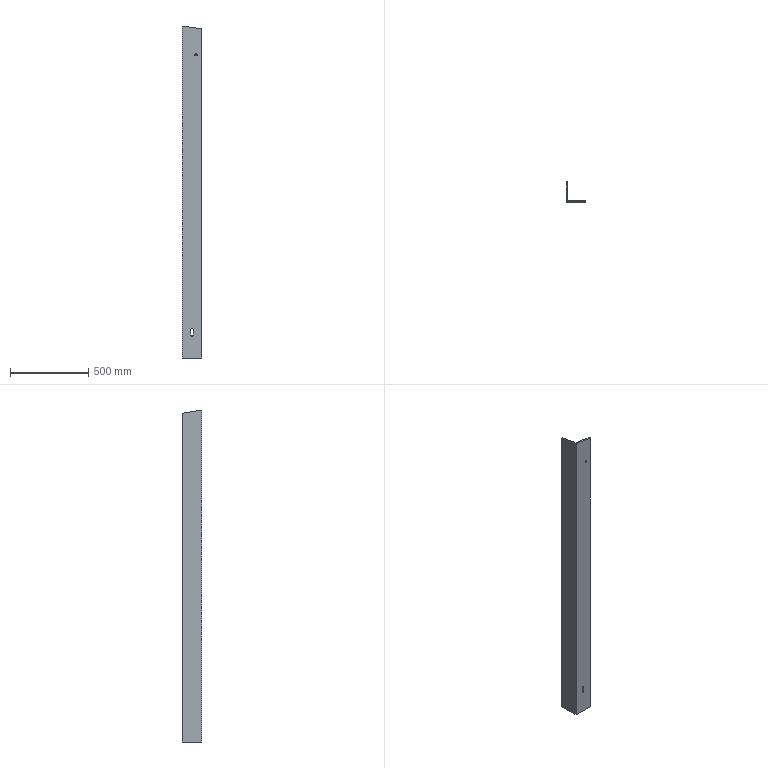Part | SolidWorks | features ICE 2, Extrusion 1 | 1 solid | 15 faces | box 127 x 127 x 2128 mm | volume 4129005 mm3 | plane 11 | cylinder 4 | commonest cylinder face diameters 14.287 x4
STEP:
#1=CARTESIAN_POINT('',(96.044,0.,879.284));
#2=VERTEX_POINT('',#1);
#3=CARTESIAN_POINT('',(81.756,0.,879.284));
#4=VERTEX_POINT('',#3);
#5=CARTESIAN_POINT('',(88.9,0.,879.284));
#6=DIRECTION('',(0.,1.,0.));
#7=DIRECTION('',(0.,0.,1.));
#8=AXIS2_PLACEMENT_3D('',#5,#6,#7);
#9=CIRCLE('',#8,7.144);
#10=EDGE_CURVE('',#2,#4,#9,.T.);
#11=ORIENTED_EDGE('',*,*,#10,.F.);
#12=CARTESIAN_POINT('',(96.044,7.937,879.284));
#13=VERTEX_POINT('',#12);
#14=CARTESIAN_POINT('',(96.044,-242.062,879.284));
#15=DIRECTION('',(0.,1.,0.));
#16=VECTOR('',#15,1000.);
#17=LINE('',#14,#16);
#18=EDGE_CURVE('',#2,#13,#17,.T.);
#19=ORIENTED_EDGE('',*,*,#18,.T.);
#20=CARTESIAN_POINT('',(81.756,7.937,879.284));
#21=VERTEX_POINT('',#20);
#22=CARTESIAN_POINT('',(88.9,7.937,879.284));
#23=DIRECTION('',(0.,-1.,0.));
#24=DIRECTION('',(1.,0.,0.));
#25=AXIS2_PLACEMENT_3D('',#22,#23,#24);
#26=CIRCLE('',#25,7.144);
#27=EDGE_CURVE('',#21,#13,#26,.T.);
#28=ORIENTED_EDGE('',*,*,#27,.F.);
#29=CARTESIAN_POINT('',(81.756,-242.062,879.284));
#30=DIRECTION('',(0.,1.,0.));
#31=VECTOR('',#30,1000.);
#32=LINE('',#29,#31);
#33=EDGE_CURVE('',#4,#21,#32,.T.);
#34=ORIENTED_EDGE('',*,*,#33,.F.);
#35=EDGE_LOOP('',(#11,#19,#28,#34));
#36=FACE_OUTER_BOUND('',#35,.T.);
#37=CARTESIAN_POINT('',(88.9,-242.062,879.284));
#38=DIRECTION('',(0.,1.,0.));
#39=DIRECTION('',(-1.,0.,0.));
#40=AXIS2_PLACEMENT_3D('',#37,#38,#39);
#41=CYLINDRICAL_SURFACE('',#40,7.144);
#42=ADVANCED_FACE('',(#36),#41,.F.);
#43=CARTESIAN_POINT('',(0.,127.,1042.677));
#44=VERTEX_POINT('',#43);
#45=CARTESIAN_POINT('',(0.,127.,-1063.815));
#46=VERTEX_POINT('',#45);
#47=CARTESIAN_POINT('',(0.,127.,1063.815));
#48=DIRECTION('',(0.,0.,-1.));
#49=VECTOR('',#48,1000.);
#50=LINE('',#47,#49);
#51=EDGE_CURVE('',#44,#46,#50,.T.);
#52=ORIENTED_EDGE('',*,*,#51,.F.);
#53=CARTESIAN_POINT('',(7.938,127.,1042.677));
#54=VERTEX_POINT('',#53);
#55=CARTESIAN_POINT('',(150.,127.,1042.677));
#56=DIRECTION('',(-1.,0.,0.));
#57=VECTOR('',#56,1000.);
#58=LINE('',#55,#57);
#59=EDGE_CURVE('',#54,#44,#58,.T.);
#60=ORIENTED_EDGE('',*,*,#59,.F.);
#61=CARTESIAN_POINT('',(7.938,127.,-1063.815));
#62=VERTEX_POINT('',#61);
#63=CARTESIAN_POINT('',(7.938,127.,1063.815));
#64=DIRECTION('',(0.,0.,-1.));
#65=VECTOR('',#64,1000.);
#66=LINE('',#63,#65);
#67=EDGE_CURVE('',#54,#62,#66,.T.);
#68=ORIENTED_EDGE('',*,*,#67,.T.);
#69=CARTESIAN_POINT('',(7.938,127.,-1063.815));
#70=DIRECTION('',(-1.,0.,0.));
#71=VECTOR('',#70,1000.);
#72=LINE('',#69,#71);
#73=EDGE_CURVE('',#62,#46,#72,.T.);
#74=ORIENTED_EDGE('',*,*,#73,.T.);
#75=EDGE_LOOP('',(#52,#60,#68,#74));
#76=FACE_OUTER_BOUND('',#75,.T.);
#77=CARTESIAN_POINT('',(7.938,127.,1063.815));
#78=DIRECTION('',(0.,-1.,0.));
#79=DIRECTION('',(0.,0.,-1.));
#80=AXIS2_PLACEMENT_3D('',#77,#78,#79);
#81=PLANE('',#80);
#82=ADVANCED_FACE('',(#76),#81,.F.);
#83=CARTESIAN_POINT('',(0.,0.,1063.815));
#84=VERTEX_POINT('',#83);
#85=CARTESIAN_POINT('',(0.,0.,-1063.815));
#86=VERTEX_POINT('',#85);
#87=CARTESIAN_POINT('',(0.,0.,1063.815));
#88=DIRECTION('',(0.,0.,-1.));
#89=VECTOR('',#88,1000.);
#90=LINE('',#87,#89);
#91=EDGE_CURVE('',#84,#86,#90,.T.);
#92=ORIENTED_EDGE('',*,*,#91,.F.);
#93=CARTESIAN_POINT('',(0.,0.,1063.815));
#94=DIRECTION('',(0.,-0.9864,0.1642));
#95=VECTOR('',#94,1000.);
#96=LINE('',#93,#95);
#97=EDGE_CURVE('',#44,#84,#96,.T.);
#98=ORIENTED_EDGE('',*,*,#97,.F.);
#99=ORIENTED_EDGE('',*,*,#51,.T.);
#100=CARTESIAN_POINT('',(0.,127.,-1063.815));
#101=DIRECTION('',(0.,-1.,0.));
#102=VECTOR('',#101,1000.);
#103=LINE('',#100,#102);
#104=EDGE_CURVE('',#46,#86,#103,.T.);
#105=ORIENTED_EDGE('',*,*,#104,.T.);
#106=EDGE_LOOP('',(#92,#98,#99,#105));
#107=FACE_OUTER_BOUND('',#106,.T.);
#108=CARTESIAN_POINT('',(0.,127.,1063.815));
#109=DIRECTION('',(1.,0.,0.));
#110=DIRECTION('',(0.,0.,-1.));
#111=AXIS2_PLACEMENT_3D('',#108,#109,#110);
#112=PLANE('',#111);
#113=ADVANCED_FACE('',(#107),#112,.F.);
#114=CARTESIAN_POINT('',(88.9,0.,879.284));
#115=DIRECTION('',(0.,1.,0.));
#116=DIRECTION('',(0.,0.,1.));
#117=AXIS2_PLACEMENT_3D('',#114,#115,#116);
#118=CIRCLE('',#117,7.144);
#119=EDGE_CURVE('',#4,#2,#118,.T.);
#120=ORIENTED_EDGE('',*,*,#119,.T.);
#121=ORIENTED_EDGE('',*,*,#10,.T.);
#122=EDGE_LOOP('',(#120,#121));
#123=FACE_BOUND('',#122,.T.);
#124=CARTESIAN_POINT('',(70.644,0.,-880.459));
#125=VERTEX_POINT('',#124);
#126=CARTESIAN_POINT('',(70.644,0.,-916.972));
#127=VERTEX_POINT('',#126);
#128=CARTESIAN_POINT('',(70.644,0.,1063.815));
#129=DIRECTION('',(0.,0.,-1.));
#130=VECTOR('',#129,1000.);
#131=LINE('',#128,#130);
#132=EDGE_CURVE('',#125,#127,#131,.T.);
#133=ORIENTED_EDGE('',*,*,#132,.T.);
#134=CARTESIAN_POINT('',(56.356,0.,-916.972));
#135=VERTEX_POINT('',#134);
#136=CARTESIAN_POINT('',(63.5,0.,-916.972));
#137=DIRECTION('',(0.,1.,0.));
#138=DIRECTION('',(0.,0.,1.));
#139=AXIS2_PLACEMENT_3D('',#136,#137,#138);
#140=CIRCLE('',#139,7.144);
#141=EDGE_CURVE('',#127,#135,#140,.T.);
#142=ORIENTED_EDGE('',*,*,#141,.T.);
#143=CARTESIAN_POINT('',(56.356,0.,-880.459));
#144=VERTEX_POINT('',#143);
#145=CARTESIAN_POINT('',(56.356,0.,1063.815));
#146=DIRECTION('',(0.,0.,1.));
#147=VECTOR('',#146,1000.);
#148=LINE('',#145,#147);
#149=EDGE_CURVE('',#135,#144,#148,.T.);
#150=ORIENTED_EDGE('',*,*,#149,.T.);
#151=CARTESIAN_POINT('',(63.5,0.,-880.459));
#152=DIRECTION('',(0.,1.,0.));
#153=DIRECTION('',(0.,0.,1.));
#154=AXIS2_PLACEMENT_3D('',#151,#152,#153);
#155=CIRCLE('',#154,7.144);
#156=EDGE_CURVE('',#144,#125,#155,.T.);
#157=ORIENTED_EDGE('',*,*,#156,.T.);
#158=EDGE_LOOP('',(#133,#142,#150,#157));
#159=FACE_BOUND('',#158,.T.);
#160=CARTESIAN_POINT('',(127.,0.,1045.56));
#161=VERTEX_POINT('',#160);
#162=CARTESIAN_POINT('',(127.,0.,-1063.815));
#163=VERTEX_POINT('',#162);
#164=CARTESIAN_POINT('',(127.,0.,1063.815));
#165=DIRECTION('',(0.,0.,-1.));
#166=VECTOR('',#165,1000.);
#167=LINE('',#164,#166);
#168=EDGE_CURVE('',#161,#163,#167,.T.);
#169=ORIENTED_EDGE('',*,*,#168,.F.);
#170=CARTESIAN_POINT('',(0.,0.,1063.815));
#171=DIRECTION('',(-0.9898,0.,0.1423));
#172=VECTOR('',#171,1000.);
#173=LINE('',#170,#172);
#174=EDGE_CURVE('',#161,#84,#173,.T.);
#175=ORIENTED_EDGE('',*,*,#174,.T.);
#176=ORIENTED_EDGE('',*,*,#91,.T.);
#177=CARTESIAN_POINT('',(0.,0.,-1063.815));
#178=DIRECTION('',(1.,0.,0.));
#179=VECTOR('',#178,1000.);
#180=LINE('',#177,#179);
#181=EDGE_CURVE('',#86,#163,#180,.T.);
#182=ORIENTED_EDGE('',*,*,#181,.T.);
#183=EDGE_LOOP('',(#169,#175,#176,#182));
#184=FACE_OUTER_BOUND('',#183,.T.);
#185=CARTESIAN_POINT('',(0.,0.,1063.815));
#186=DIRECTION('',(0.,1.,0.));
#187=DIRECTION('',(0.,0.,1.));
#188=AXIS2_PLACEMENT_3D('',#185,#186,#187);
#189=PLANE('',#188);
#190=ADVANCED_FACE('',(#123,#159,#184),#189,.F.);
#191=CARTESIAN_POINT('',(127.,7.937,1045.56));
#192=VERTEX_POINT('',#191);
#193=CARTESIAN_POINT('',(127.,7.938,-1063.815));
#194=VERTEX_POINT('',#193);
#195=CARTESIAN_POINT('',(127.,7.938,1063.815));
#196=DIRECTION('',(0.,0.,-1.));
#197=VECTOR('',#196,1000.);
#198=LINE('',#195,#197);
#199=EDGE_CURVE('',#192,#194,#198,.T.);
#200=ORIENTED_EDGE('',*,*,#199,.F.);
#201=CARTESIAN_POINT('',(127.,-242.062,1045.56));
#202=DIRECTION('',(0.,1.,0.));
#203=VECTOR('',#202,1000.);
#204=LINE('',#201,#203);
#205=EDGE_CURVE('',#161,#192,#204,.T.);
#206=ORIENTED_EDGE('',*,*,#205,.F.);
#207=ORIENTED_EDGE('',*,*,#168,.T.);
#208=CARTESIAN_POINT('',(127.,0.,-1063.815));
#209=DIRECTION('',(0.,1.,0.));
#210=VECTOR('',#209,1000.);
#211=LINE('',#208,#210);
#212=EDGE_CURVE('',#163,#194,#211,.T.);
#213=ORIENTED_EDGE('',*,*,#212,.T.);
#214=EDGE_LOOP('',(#200,#206,#207,#213));
#215=FACE_OUTER_BOUND('',#214,.T.);
#216=CARTESIAN_POINT('',(127.,0.,1063.815));
#217=DIRECTION('',(-1.,0.,0.));
#218=DIRECTION('',(0.,0.,1.));
#219=AXIS2_PLACEMENT_3D('',#216,#217,#218);
#220=PLANE('',#219);
#221=ADVANCED_FACE('',(#215),#220,.F.);
#222=ORIENTED_EDGE('',*,*,#27,.T.);
#223=CARTESIAN_POINT('',(88.9,7.937,879.284));
#224=DIRECTION('',(0.,-1.,0.));
#225=DIRECTION('',(1.,0.,0.));
#226=AXIS2_PLACEMENT_3D('',#223,#224,#225);
#227=CIRCLE('',#226,7.144);
#228=EDGE_CURVE('',#13,#21,#227,.T.);
#229=ORIENTED_EDGE('',*,*,#228,.T.);
#230=EDGE_LOOP('',(#222,#229));
#231=FACE_BOUND('',#230,.T.);
#232=CARTESIAN_POINT('',(56.356,7.937,-880.459));
#233=VERTEX_POINT('',#232);
#234=CARTESIAN_POINT('',(56.356,7.937,-916.972));
#235=VERTEX_POINT('',#234);
#236=CARTESIAN_POINT('',(56.356,7.937,1063.815));
#237=DIRECTION('',(0.,0.,-1.));
#238=VECTOR('',#237,1000.);
#239=LINE('',#236,#238);
#240=EDGE_CURVE('',#233,#235,#239,.T.);
#241=ORIENTED_EDGE('',*,*,#240,.T.);
#242=CARTESIAN_POINT('',(70.644,7.937,-916.972));
#243=VERTEX_POINT('',#242);
#244=CARTESIAN_POINT('',(63.5,7.937,-916.972));
#245=DIRECTION('',(0.,-1.,0.));
#246=DIRECTION('',(1.,0.,0.));
#247=AXIS2_PLACEMENT_3D('',#244,#245,#246);
#248=CIRCLE('',#247,7.144);
#249=EDGE_CURVE('',#235,#243,#248,.T.);
#250=ORIENTED_EDGE('',*,*,#249,.T.);
#251=CARTESIAN_POINT('',(70.644,7.937,-880.459));
#252=VERTEX_POINT('',#251);
#253=CARTESIAN_POINT('',(70.644,7.938,1063.815));
#254=DIRECTION('',(0.,0.,1.));
#255=VECTOR('',#254,1000.);
#256=LINE('',#253,#255);
#257=EDGE_CURVE('',#243,#252,#256,.T.);
#258=ORIENTED_EDGE('',*,*,#257,.T.);
#259=CARTESIAN_POINT('',(63.5,7.937,-880.459));
#260=DIRECTION('',(0.,-1.,0.));
#261=DIRECTION('',(1.,0.,0.));
#262=AXIS2_PLACEMENT_3D('',#259,#260,#261);
#263=CIRCLE('',#262,7.144);
#264=EDGE_CURVE('',#252,#233,#263,.T.);
#265=ORIENTED_EDGE('',*,*,#264,.T.);
#266=EDGE_LOOP('',(#241,#250,#258,#265));
#267=FACE_BOUND('',#266,.T.);
#268=CARTESIAN_POINT('',(7.938,7.937,1062.494));
#269=VERTEX_POINT('',#268);
#270=CARTESIAN_POINT('',(9.191,7.937,1062.494));
#271=VERTEX_POINT('',#270);
#272=CARTESIAN_POINT('',(127.,7.938,1062.494));
#273=DIRECTION('',(1.,0.,0.));
#274=VECTOR('',#273,1000.);
#275=LINE('',#272,#274);
#276=EDGE_CURVE('',#269,#271,#275,.T.);
#277=ORIENTED_EDGE('',*,*,#276,.T.);
#278=CARTESIAN_POINT('',(124.429,7.938,1045.929));
#279=DIRECTION('',(0.9898,0.,-0.1423));
#280=VECTOR('',#279,1000.);
#281=LINE('',#278,#280);
#282=EDGE_CURVE('',#271,#192,#281,.T.);
#283=ORIENTED_EDGE('',*,*,#282,.T.);
#284=ORIENTED_EDGE('',*,*,#199,.T.);
#285=CARTESIAN_POINT('',(7.938,7.937,-1063.815));
#286=VERTEX_POINT('',#285);
#287=CARTESIAN_POINT('',(127.,7.938,-1063.815));
#288=DIRECTION('',(-1.,0.,0.));
#289=VECTOR('',#288,1000.);
#290=LINE('',#287,#289);
#291=EDGE_CURVE('',#194,#286,#290,.T.);
#292=ORIENTED_EDGE('',*,*,#291,.T.);
#293=CARTESIAN_POINT('',(7.938,7.937,1063.815));
#294=DIRECTION('',(0.,0.,-1.));
#295=VECTOR('',#294,1000.);
#296=LINE('',#293,#295);
#297=EDGE_CURVE('',#269,#286,#296,.T.);
#298=ORIENTED_EDGE('',*,*,#297,.F.);
#299=EDGE_LOOP('',(#277,#283,#284,#292,#298));
#300=FACE_OUTER_BOUND('',#299,.T.);
#301=CARTESIAN_POINT('',(127.,7.938,1063.815));
#302=DIRECTION('',(0.,-1.,0.));
#303=DIRECTION('',(1.,0.,0.));
#304=AXIS2_PLACEMENT_3D('',#301,#302,#303);
#305=PLANE('',#304);
#306=ADVANCED_FACE('',(#231,#267,#300),#305,.F.);
#307=ORIENTED_EDGE('',*,*,#67,.F.);
#308=CARTESIAN_POINT('',(7.938,7.724,1062.53));
#309=DIRECTION('',(0.,-0.9864,0.1642));
#310=VECTOR('',#309,1000.);
#311=LINE('',#308,#310);
#312=EDGE_CURVE('',#54,#269,#311,.T.);
#313=ORIENTED_EDGE('',*,*,#312,.T.);
#314=ORIENTED_EDGE('',*,*,#297,.T.);
#315=CARTESIAN_POINT('',(7.938,7.937,-1063.815));
#316=DIRECTION('',(0.,1.,0.));
#317=VECTOR('',#316,1000.);
#318=LINE('',#315,#317);
#319=EDGE_CURVE('',#286,#62,#318,.T.);
#320=ORIENTED_EDGE('',*,*,#319,.T.);
#321=EDGE_LOOP('',(#307,#313,#314,#320));
#322=FACE_OUTER_BOUND('',#321,.T.);
#323=CARTESIAN_POINT('',(7.938,7.937,1063.815));
#324=DIRECTION('',(-1.,0.,0.));
#325=DIRECTION('',(0.,0.,1.));
#326=AXIS2_PLACEMENT_3D('',#323,#324,#325);
#327=PLANE('',#326);
#328=ADVANCED_FACE('',(#322),#327,.F.);
#329=ORIENTED_EDGE('',*,*,#73,.F.);
#330=ORIENTED_EDGE('',*,*,#319,.F.);
#331=ORIENTED_EDGE('',*,*,#291,.F.);
#332=ORIENTED_EDGE('',*,*,#212,.F.);
#333=ORIENTED_EDGE('',*,*,#181,.F.);
#334=ORIENTED_EDGE('',*,*,#104,.F.);
#335=EDGE_LOOP('',(#329,#330,#331,#332,#333,#334));
#336=FACE_OUTER_BOUND('',#335,.T.);
#337=CARTESIAN_POINT('',(0.,127.,-1063.815));
#338=DIRECTION('',(0.,0.,1.));
#339=DIRECTION('',(1.,0.,0.));
#340=AXIS2_PLACEMENT_3D('',#337,#338,#339);
#341=PLANE('',#340);
#342=ADVANCED_FACE('',(#336),#341,.F.);
#343=ORIENTED_EDGE('',*,*,#97,.T.);
#344=CARTESIAN_POINT('',(84.913,73.333,1051.61));
#345=DIRECTION('',(0.7524,0.6498,-0.1082));
#346=VECTOR('',#345,1000.);
#347=LINE('',#344,#346);
#348=EDGE_CURVE('',#84,#271,#347,.T.);
#349=ORIENTED_EDGE('',*,*,#348,.T.);
#350=ORIENTED_EDGE('',*,*,#276,.F.);
#351=ORIENTED_EDGE('',*,*,#312,.F.);
#352=ORIENTED_EDGE('',*,*,#59,.T.);
#353=EDGE_LOOP('',(#343,#349,#350,#351,#352));
#354=FACE_OUTER_BOUND('',#353,.T.);
#355=CARTESIAN_POINT('',(150.,0.,1063.815));
#356=DIRECTION('',(0.,-0.1642,-0.9864));
#357=DIRECTION('',(0.,0.9864,-0.1642));
#358=AXIS2_PLACEMENT_3D('',#355,#356,#357);
#359=PLANE('',#358);
#360=ADVANCED_FACE('',(#354),#359,.F.);
#361=ORIENTED_EDGE('',*,*,#205,.T.);
#362=ORIENTED_EDGE('',*,*,#282,.F.);
#363=ORIENTED_EDGE('',*,*,#348,.F.);
#364=ORIENTED_EDGE('',*,*,#174,.F.);
#365=EDGE_LOOP('',(#361,#362,#363,#364));
#366=FACE_OUTER_BOUND('',#365,.T.);
#367=CARTESIAN_POINT('',(127.,-242.062,1045.56));
#368=DIRECTION('',(-0.1423,0.,-0.9898));
#369=DIRECTION('',(-0.9898,0.,0.1423));
#370=AXIS2_PLACEMENT_3D('',#367,#368,#369);
#371=PLANE('',#370);
#372=ADVANCED_FACE('',(#366),#371,.F.);
#373=CARTESIAN_POINT('',(70.644,-242.062,-916.972));
#374=DIRECTION('',(0.,1.,0.));
#375=VECTOR('',#374,1000.);
#376=LINE('',#373,#375);
#377=EDGE_CURVE('',#127,#243,#376,.T.);
#378=ORIENTED_EDGE('',*,*,#377,.T.);
#379=ORIENTED_EDGE('',*,*,#249,.F.);
#380=CARTESIAN_POINT('',(56.356,-242.062,-916.972));
#381=DIRECTION('',(0.,1.,0.));
#382=VECTOR('',#381,1000.);
#383=LINE('',#380,#382);
#384=EDGE_CURVE('',#135,#235,#383,.T.);
#385=ORIENTED_EDGE('',*,*,#384,.F.);
#386=ORIENTED_EDGE('',*,*,#141,.F.);
#387=EDGE_LOOP('',(#378,#379,#385,#386));
#388=FACE_OUTER_BOUND('',#387,.T.);
#389=CARTESIAN_POINT('',(63.5,-242.062,-916.972));
#390=DIRECTION('',(0.,1.,0.));
#391=DIRECTION('',(-1.,0.,0.));
#392=AXIS2_PLACEMENT_3D('',#389,#390,#391);
#393=CYLINDRICAL_SURFACE('',#392,7.144);
#394=ADVANCED_FACE('',(#388),#393,.F.);
#395=CARTESIAN_POINT('',(70.644,-242.062,-880.459));
#396=DIRECTION('',(0.,1.,0.));
#397=VECTOR('',#396,1000.);
#398=LINE('',#395,#397);
#399=EDGE_CURVE('',#125,#252,#398,.T.);
#400=ORIENTED_EDGE('',*,*,#399,.T.);
#401=ORIENTED_EDGE('',*,*,#257,.F.);
#402=ORIENTED_EDGE('',*,*,#377,.F.);
#403=ORIENTED_EDGE('',*,*,#132,.F.);
#404=EDGE_LOOP('',(#400,#401,#402,#403));
#405=FACE_OUTER_BOUND('',#404,.T.);
#406=CARTESIAN_POINT('',(70.644,-242.062,-916.972));
#407=DIRECTION('',(1.,0.,0.));
#408=DIRECTION('',(0.,1.,0.));
#409=AXIS2_PLACEMENT_3D('',#406,#407,#408);
#410=PLANE('',#409);
#411=ADVANCED_FACE('',(#405),#410,.F.);
#412=CARTESIAN_POINT('',(56.356,-242.062,-880.459));
#413=DIRECTION('',(0.,1.,0.));
#414=VECTOR('',#413,1000.);
#415=LINE('',#412,#414);
#416=EDGE_CURVE('',#144,#233,#415,.T.);
#417=ORIENTED_EDGE('',*,*,#416,.T.);
#418=ORIENTED_EDGE('',*,*,#264,.F.);
#419=ORIENTED_EDGE('',*,*,#399,.F.);
#420=ORIENTED_EDGE('',*,*,#156,.F.);
#421=EDGE_LOOP('',(#417,#418,#419,#420));
#422=FACE_OUTER_BOUND('',#421,.T.);
#423=CARTESIAN_POINT('',(63.5,-242.062,-880.459));
#424=DIRECTION('',(0.,1.,0.));
#425=DIRECTION('',(-1.,0.,0.));
#426=AXIS2_PLACEMENT_3D('',#423,#424,#425);
#427=CYLINDRICAL_SURFACE('',#426,7.144);
#428=ADVANCED_FACE('',(#422),#427,.F.);
#429=ORIENTED_EDGE('',*,*,#384,.T.);
#430=ORIENTED_EDGE('',*,*,#240,.F.);
#431=ORIENTED_EDGE('',*,*,#416,.F.);
#432=ORIENTED_EDGE('',*,*,#149,.F.);
#433=EDGE_LOOP('',(#429,#430,#431,#432));
#434=FACE_OUTER_BOUND('',#433,.T.);
#435=CARTESIAN_POINT('',(56.356,-242.062,-916.972));
#436=DIRECTION('',(-1.,0.,0.));
#437=DIRECTION('',(0.,0.,1.));
#438=AXIS2_PLACEMENT_3D('',#435,#436,#437);
#439=PLANE('',#438);
#440=ADVANCED_FACE('',(#434),#439,.F.);
#441=ORIENTED_EDGE('',*,*,#18,.F.);
#442=ORIENTED_EDGE('',*,*,#119,.F.);
#443=ORIENTED_EDGE('',*,*,#33,.T.);
#444=ORIENTED_EDGE('',*,*,#228,.F.);
#445=EDGE_LOOP('',(#441,#442,#443,#444));
#446=FACE_OUTER_BOUND('',#445,.T.);
#447=CARTESIAN_POINT('',(88.9,-242.062,879.284));
#448=DIRECTION('',(0.,1.,0.));
#449=DIRECTION('',(-1.,0.,0.));
#450=AXIS2_PLACEMENT_3D('',#447,#448,#449);
#451=CYLINDRICAL_SURFACE('',#450,7.144);
#452=ADVANCED_FACE('',(#446),#451,.F.);
#453=CLOSED_SHELL('',(#42,#82,#113,#190,#221,#306,#328,#342,#360,#372,#394,#411,#428,#440,#452));
#454=MANIFOLD_SOLID_BREP('',#453);
#455=CARTESIAN_POINT('',(0.,0.,0.));
#456=DIRECTION('',(0.,0.,1.));
#457=DIRECTION('',(1.,0.,0.));
#458=AXIS2_PLACEMENT_3D('',#455,#456,#457);
#459=(LENGTH_UNIT()NAMED_UNIT(*)SI_UNIT(.MILLI.,.METRE.));
#460=UNCERTAINTY_MEASURE_WITH_UNIT(LENGTH_MEASURE(0.00001),#459,'','');
#461=(NAMED_UNIT(*)PLANE_ANGLE_UNIT()SI_UNIT($,.RADIAN.));
#462=(NAMED_UNIT(*)SI_UNIT($,.STERADIAN.)SOLID_ANGLE_UNIT());
#463=(GEOMETRIC_REPRESENTATION_CONTEXT(3)GLOBAL_UNCERTAINTY_ASSIGNED_CONTEXT((#460))GLOBAL_UNIT_ASSIGNED_CONTEXT((#459,#461,#462))REPRESENTATION_CONTEXT('',''));
#464=ADVANCED_BREP_SHAPE_REPRESENTATION('',(#454,#458),#463);